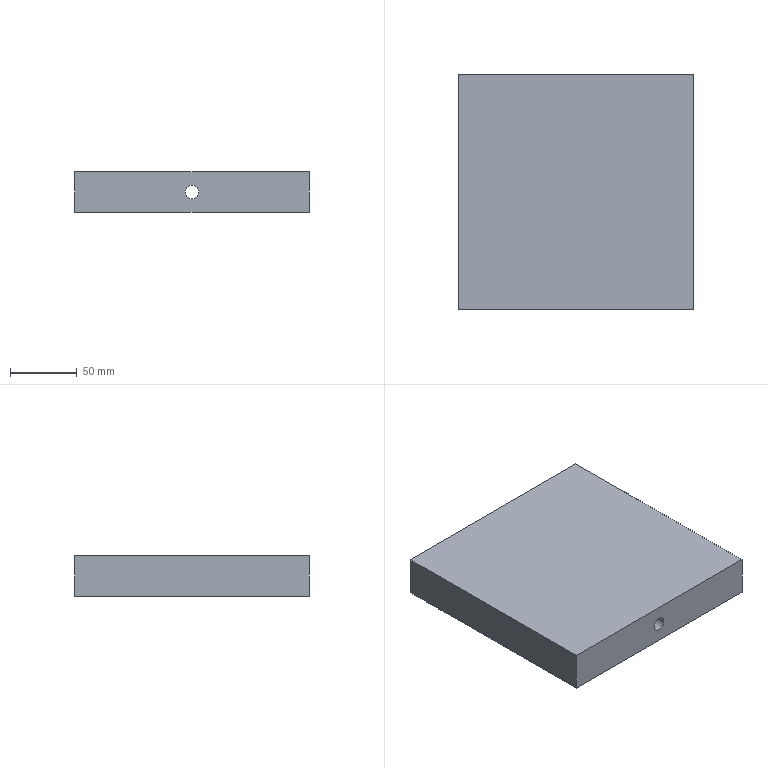Part | SolidWorks | features Extrusion 1, ICE 1 | 1 solid | 8 faces | box 176 x 176 x 30 mm | volume 915151 mm3 | plane 6 | cylinder 2 | commonest cylinder face diameters 10.11 x2
STEP:
#1=CARTESIAN_POINT('',(5.055,-88.,15.));
#2=VERTEX_POINT('',#1);
#3=CARTESIAN_POINT('',(-5.055,-88.,15.));
#4=VERTEX_POINT('',#3);
#5=CARTESIAN_POINT('',(0.,-88.,15.));
#6=DIRECTION('',(0.,1.,0.));
#7=DIRECTION('',(-1.,0.,0.));
#8=AXIS2_PLACEMENT_3D('',#5,#6,#7);
#9=CIRCLE('',#8,5.055);
#10=EDGE_CURVE('',#2,#4,#9,.T.);
#11=ORIENTED_EDGE('',*,*,#10,.F.);
#12=CARTESIAN_POINT('',(5.055,88.,15.));
#13=VERTEX_POINT('',#12);
#14=CARTESIAN_POINT('',(5.055,-88.,15.));
#15=DIRECTION('',(0.,1.,0.));
#16=VECTOR('',#15,1000.);
#17=LINE('',#14,#16);
#18=EDGE_CURVE('',#2,#13,#17,.T.);
#19=ORIENTED_EDGE('',*,*,#18,.T.);
#20=CARTESIAN_POINT('',(-5.055,88.,15.));
#21=VERTEX_POINT('',#20);
#22=CARTESIAN_POINT('',(0.,88.,15.));
#23=DIRECTION('',(0.,1.,0.));
#24=DIRECTION('',(-1.,0.,0.));
#25=AXIS2_PLACEMENT_3D('',#22,#23,#24);
#26=CIRCLE('',#25,5.055);
#27=EDGE_CURVE('',#13,#21,#26,.T.);
#28=ORIENTED_EDGE('',*,*,#27,.T.);
#29=CARTESIAN_POINT('',(-5.055,-88.,15.));
#30=DIRECTION('',(0.,1.,0.));
#31=VECTOR('',#30,1000.);
#32=LINE('',#29,#31);
#33=EDGE_CURVE('',#4,#21,#32,.T.);
#34=ORIENTED_EDGE('',*,*,#33,.F.);
#35=EDGE_LOOP('',(#11,#19,#28,#34));
#36=FACE_OUTER_BOUND('',#35,.T.);
#37=CARTESIAN_POINT('',(0.,-88.,15.));
#38=DIRECTION('',(0.,1.,0.));
#39=DIRECTION('',(-1.,0.,0.));
#40=AXIS2_PLACEMENT_3D('',#37,#38,#39);
#41=CYLINDRICAL_SURFACE('',#40,5.055);
#42=ADVANCED_FACE('',(#36),#41,.F.);
#43=CARTESIAN_POINT('',(-88.,88.,0.));
#44=VERTEX_POINT('',#43);
#45=CARTESIAN_POINT('',(-88.,-88.,0.));
#46=VERTEX_POINT('',#45);
#47=CARTESIAN_POINT('',(-88.,88.,0.));
#48=DIRECTION('',(0.,-1.,0.));
#49=VECTOR('',#48,1000.);
#50=LINE('',#47,#49);
#51=EDGE_CURVE('',#44,#46,#50,.T.);
#52=ORIENTED_EDGE('',*,*,#51,.T.);
#53=CARTESIAN_POINT('',(-88.,-88.,30.));
#54=VERTEX_POINT('',#53);
#55=CARTESIAN_POINT('',(-88.,-88.,30.));
#56=DIRECTION('',(0.,0.,-1.));
#57=VECTOR('',#56,1000.);
#58=LINE('',#55,#57);
#59=EDGE_CURVE('',#54,#46,#58,.T.);
#60=ORIENTED_EDGE('',*,*,#59,.F.);
#61=CARTESIAN_POINT('',(-88.,88.,30.));
#62=VERTEX_POINT('',#61);
#63=CARTESIAN_POINT('',(-88.,88.,30.));
#64=DIRECTION('',(0.,-1.,0.));
#65=VECTOR('',#64,1000.);
#66=LINE('',#63,#65);
#67=EDGE_CURVE('',#62,#54,#66,.T.);
#68=ORIENTED_EDGE('',*,*,#67,.F.);
#69=CARTESIAN_POINT('',(-88.,88.,30.));
#70=DIRECTION('',(0.,0.,-1.));
#71=VECTOR('',#70,1000.);
#72=LINE('',#69,#71);
#73=EDGE_CURVE('',#62,#44,#72,.T.);
#74=ORIENTED_EDGE('',*,*,#73,.T.);
#75=EDGE_LOOP('',(#52,#60,#68,#74));
#76=FACE_OUTER_BOUND('',#75,.T.);
#77=CARTESIAN_POINT('',(-88.,88.,30.));
#78=DIRECTION('',(1.,0.,0.));
#79=DIRECTION('',(0.,1.,0.));
#80=AXIS2_PLACEMENT_3D('',#77,#78,#79);
#81=PLANE('',#80);
#82=ADVANCED_FACE('',(#76),#81,.F.);
#83=CARTESIAN_POINT('',(0.,-88.,15.));
#84=DIRECTION('',(0.,1.,0.));
#85=DIRECTION('',(-1.,0.,0.));
#86=AXIS2_PLACEMENT_3D('',#83,#84,#85);
#87=CIRCLE('',#86,5.055);
#88=EDGE_CURVE('',#4,#2,#87,.T.);
#89=ORIENTED_EDGE('',*,*,#88,.T.);
#90=ORIENTED_EDGE('',*,*,#10,.T.);
#91=EDGE_LOOP('',(#89,#90));
#92=FACE_BOUND('',#91,.T.);
#93=CARTESIAN_POINT('',(88.,-88.,0.));
#94=VERTEX_POINT('',#93);
#95=CARTESIAN_POINT('',(88.,-88.,0.));
#96=DIRECTION('',(1.,0.,0.));
#97=VECTOR('',#96,1000.);
#98=LINE('',#95,#97);
#99=EDGE_CURVE('',#46,#94,#98,.T.);
#100=ORIENTED_EDGE('',*,*,#99,.T.);
#101=CARTESIAN_POINT('',(88.,-88.,30.));
#102=VERTEX_POINT('',#101);
#103=CARTESIAN_POINT('',(88.,-88.,30.));
#104=DIRECTION('',(0.,0.,-1.));
#105=VECTOR('',#104,1000.);
#106=LINE('',#103,#105);
#107=EDGE_CURVE('',#102,#94,#106,.T.);
#108=ORIENTED_EDGE('',*,*,#107,.F.);
#109=CARTESIAN_POINT('',(88.,-88.,30.));
#110=DIRECTION('',(1.,0.,0.));
#111=VECTOR('',#110,1000.);
#112=LINE('',#109,#111);
#113=EDGE_CURVE('',#54,#102,#112,.T.);
#114=ORIENTED_EDGE('',*,*,#113,.F.);
#115=ORIENTED_EDGE('',*,*,#59,.T.);
#116=EDGE_LOOP('',(#100,#108,#114,#115));
#117=FACE_OUTER_BOUND('',#116,.T.);
#118=CARTESIAN_POINT('',(88.,-88.,30.));
#119=DIRECTION('',(0.,1.,0.));
#120=DIRECTION('',(-1.,0.,0.));
#121=AXIS2_PLACEMENT_3D('',#118,#119,#120);
#122=PLANE('',#121);
#123=ADVANCED_FACE('',(#92,#117),#122,.F.);
#124=CARTESIAN_POINT('',(88.,88.,0.));
#125=VERTEX_POINT('',#124);
#126=CARTESIAN_POINT('',(88.,88.,0.));
#127=DIRECTION('',(0.,1.,0.));
#128=VECTOR('',#127,1000.);
#129=LINE('',#126,#128);
#130=EDGE_CURVE('',#94,#125,#129,.T.);
#131=ORIENTED_EDGE('',*,*,#130,.T.);
#132=CARTESIAN_POINT('',(88.,88.,30.));
#133=VERTEX_POINT('',#132);
#134=CARTESIAN_POINT('',(88.,88.,30.));
#135=DIRECTION('',(0.,0.,-1.));
#136=VECTOR('',#135,1000.);
#137=LINE('',#134,#136);
#138=EDGE_CURVE('',#133,#125,#137,.T.);
#139=ORIENTED_EDGE('',*,*,#138,.F.);
#140=CARTESIAN_POINT('',(88.,88.,30.));
#141=DIRECTION('',(0.,1.,0.));
#142=VECTOR('',#141,1000.);
#143=LINE('',#140,#142);
#144=EDGE_CURVE('',#102,#133,#143,.T.);
#145=ORIENTED_EDGE('',*,*,#144,.F.);
#146=ORIENTED_EDGE('',*,*,#107,.T.);
#147=EDGE_LOOP('',(#131,#139,#145,#146));
#148=FACE_OUTER_BOUND('',#147,.T.);
#149=CARTESIAN_POINT('',(88.,88.,30.));
#150=DIRECTION('',(-1.,0.,0.));
#151=DIRECTION('',(0.,-1.,0.));
#152=AXIS2_PLACEMENT_3D('',#149,#150,#151);
#153=PLANE('',#152);
#154=ADVANCED_FACE('',(#148),#153,.F.);
#155=CARTESIAN_POINT('',(0.,88.,15.));
#156=DIRECTION('',(0.,1.,0.));
#157=DIRECTION('',(-1.,0.,0.));
#158=AXIS2_PLACEMENT_3D('',#155,#156,#157);
#159=CIRCLE('',#158,5.055);
#160=EDGE_CURVE('',#21,#13,#159,.T.);
#161=ORIENTED_EDGE('',*,*,#160,.F.);
#162=ORIENTED_EDGE('',*,*,#27,.F.);
#163=EDGE_LOOP('',(#161,#162));
#164=FACE_BOUND('',#163,.T.);
#165=CARTESIAN_POINT('',(88.,88.,0.));
#166=DIRECTION('',(-1.,0.,0.));
#167=VECTOR('',#166,1000.);
#168=LINE('',#165,#167);
#169=EDGE_CURVE('',#125,#44,#168,.T.);
#170=ORIENTED_EDGE('',*,*,#169,.T.);
#171=ORIENTED_EDGE('',*,*,#73,.F.);
#172=CARTESIAN_POINT('',(88.,88.,30.));
#173=DIRECTION('',(-1.,0.,0.));
#174=VECTOR('',#173,1000.);
#175=LINE('',#172,#174);
#176=EDGE_CURVE('',#133,#62,#175,.T.);
#177=ORIENTED_EDGE('',*,*,#176,.F.);
#178=ORIENTED_EDGE('',*,*,#138,.T.);
#179=EDGE_LOOP('',(#170,#171,#177,#178));
#180=FACE_OUTER_BOUND('',#179,.T.);
#181=CARTESIAN_POINT('',(88.,88.,30.));
#182=DIRECTION('',(0.,-1.,0.));
#183=DIRECTION('',(1.,0.,0.));
#184=AXIS2_PLACEMENT_3D('',#181,#182,#183);
#185=PLANE('',#184);
#186=ADVANCED_FACE('',(#164,#180),#185,.F.);
#187=ORIENTED_EDGE('',*,*,#67,.T.);
#188=ORIENTED_EDGE('',*,*,#113,.T.);
#189=ORIENTED_EDGE('',*,*,#144,.T.);
#190=ORIENTED_EDGE('',*,*,#176,.T.);
#191=EDGE_LOOP('',(#187,#188,#189,#190));
#192=FACE_OUTER_BOUND('',#191,.T.);
#193=CARTESIAN_POINT('',(0.,0.,30.));
#194=DIRECTION('',(0.,0.,-1.));
#195=DIRECTION('',(-1.,0.,0.));
#196=AXIS2_PLACEMENT_3D('',#193,#194,#195);
#197=PLANE('',#196);
#198=ADVANCED_FACE('',(#192),#197,.F.);
#199=ORIENTED_EDGE('',*,*,#51,.F.);
#200=ORIENTED_EDGE('',*,*,#169,.F.);
#201=ORIENTED_EDGE('',*,*,#130,.F.);
#202=ORIENTED_EDGE('',*,*,#99,.F.);
#203=EDGE_LOOP('',(#199,#200,#201,#202));
#204=FACE_OUTER_BOUND('',#203,.T.);
#205=CARTESIAN_POINT('',(0.,0.,0.));
#206=DIRECTION('',(0.,0.,-1.));
#207=DIRECTION('',(-1.,0.,0.));
#208=AXIS2_PLACEMENT_3D('',#205,#206,#207);
#209=PLANE('',#208);
#210=ADVANCED_FACE('',(#204),#209,.T.);
#211=ORIENTED_EDGE('',*,*,#18,.F.);
#212=ORIENTED_EDGE('',*,*,#88,.F.);
#213=ORIENTED_EDGE('',*,*,#33,.T.);
#214=ORIENTED_EDGE('',*,*,#160,.T.);
#215=EDGE_LOOP('',(#211,#212,#213,#214));
#216=FACE_OUTER_BOUND('',#215,.T.);
#217=CARTESIAN_POINT('',(0.,-88.,15.));
#218=DIRECTION('',(0.,1.,0.));
#219=DIRECTION('',(-1.,0.,0.));
#220=AXIS2_PLACEMENT_3D('',#217,#218,#219);
#221=CYLINDRICAL_SURFACE('',#220,5.055);
#222=ADVANCED_FACE('',(#216),#221,.F.);
#223=CLOSED_SHELL('',(#42,#82,#123,#154,#186,#198,#210,#222));
#224=MANIFOLD_SOLID_BREP('',#223);
#225=CARTESIAN_POINT('',(0.,0.,0.));
#226=DIRECTION('',(0.,0.,1.));
#227=DIRECTION('',(1.,0.,0.));
#228=AXIS2_PLACEMENT_3D('',#225,#226,#227);
#229=(LENGTH_UNIT()NAMED_UNIT(*)SI_UNIT(.MILLI.,.METRE.));
#230=UNCERTAINTY_MEASURE_WITH_UNIT(LENGTH_MEASURE(0.00001),#229,'','');
#231=(NAMED_UNIT(*)PLANE_ANGLE_UNIT()SI_UNIT($,.RADIAN.));
#232=(NAMED_UNIT(*)SI_UNIT($,.STERADIAN.)SOLID_ANGLE_UNIT());
#233=(GEOMETRIC_REPRESENTATION_CONTEXT(3)GLOBAL_UNCERTAINTY_ASSIGNED_CONTEXT((#230))GLOBAL_UNIT_ASSIGNED_CONTEXT((#229,#231,#232))REPRESENTATION_CONTEXT('',''));
#234=ADVANCED_BREP_SHAPE_REPRESENTATION('',(#224,#228),#233);